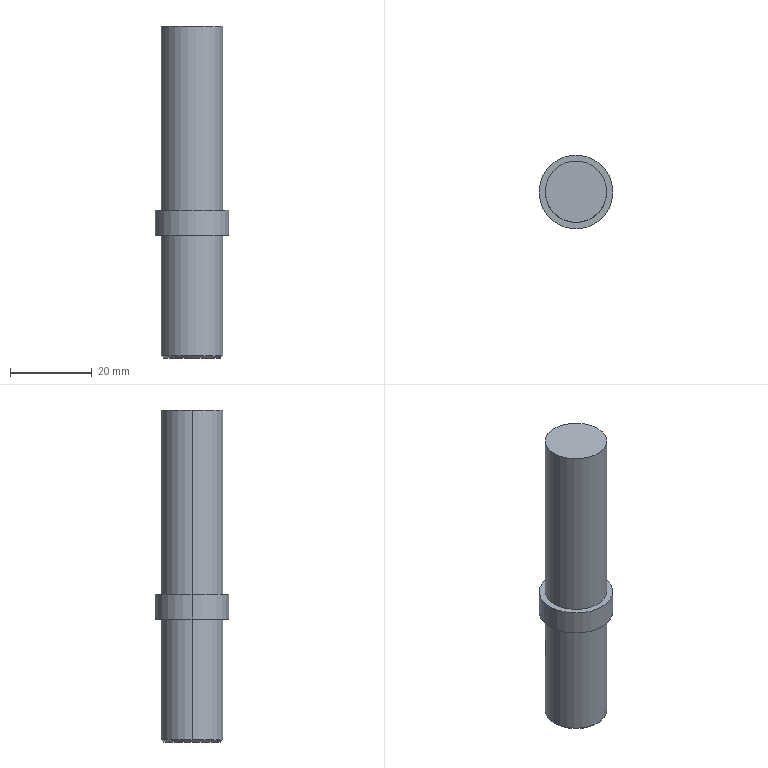Part | STEP file | 001-010-Waste driven wheel mounting shaft | 1 solid | 12 faces | box 18 x 18 x 81 mm | volume 14775 mm3 | cylinder 6 | plane 4 | cone 2 | commonest cylinder face diameters 15 x4 18 x2
STEP:
#1=CARTESIAN_POINT('',(0.,0.,0.));
#2=DIRECTION('',(0.,0.,1.));
#3=DIRECTION('',(1.,0.,0.));
#4=AXIS2_PLACEMENT_3D('',#1,#2,#3);
#5=CARTESIAN_POINT('',(-7.,0.,0.));
#6=VERTEX_POINT('',#5);
#7=CARTESIAN_POINT('',(7.,0.,0.));
#8=VERTEX_POINT('',#7);
#9=CARTESIAN_POINT('',(0.,0.,0.));
#10=DIRECTION('',(0.,0.,-1.));
#11=DIRECTION('',(1.,0.,0.));
#12=AXIS2_PLACEMENT_3D('',#9,#10,#11);
#13=CIRCLE('',#12,7.);
#14=CARTESIAN_POINT('',(0.,0.,0.5));
#15=DIRECTION('',(0.,0.,1.));
#16=DIRECTION('',(1.,0.,0.));
#17=AXIS2_PLACEMENT_3D('',#14,#15,#16);
#18=CONICAL_SURFACE('',#17,7.5,0.7854);
#19=CARTESIAN_POINT('',(6.283,-0.5));
#20=DIRECTION('',(-1.,0.));
#21=VECTOR('',#20,1.);
#22=LINE('',#19,#21);
#23=(GEOMETRIC_REPRESENTATION_CONTEXT(2)PARAMETRIC_REPRESENTATION_CONTEXT()REPRESENTATION_CONTEXT('',''));
#24=DEFINITIONAL_REPRESENTATION('',(#22),#23);
#25=PCURVE('',#18,#24);
#26=CARTESIAN_POINT('',(0.,0.,0.));
#27=DIRECTION('',(0.,0.,1.));
#28=DIRECTION('',(1.,0.,0.));
#29=AXIS2_PLACEMENT_3D('',#26,#27,#28);
#30=PLANE('',#29);
#31=CARTESIAN_POINT('',(7.,0.));
#32=CARTESIAN_POINT('',(7.,-12.124));
#33=CARTESIAN_POINT('',(-3.5,-6.062));
#34=CARTESIAN_POINT('',(-14.,0.));
#35=CARTESIAN_POINT('',(-3.5,6.062));
#36=CARTESIAN_POINT('',(7.,12.124));
#37=CARTESIAN_POINT('',(7.,0.));
#38=(BOUNDED_CURVE()B_SPLINE_CURVE(2,(#31,#32,#33,#34,#35,#36,#37),.UNSPECIFIED.,.T.,.F.)B_SPLINE_CURVE_WITH_KNOTS((1,2,2,2,2,1),(-2.094,0.,2.094,4.189,6.283,8.378),.UNSPECIFIED.)CURVE()GEOMETRIC_REPRESENTATION_ITEM()RATIONAL_B_SPLINE_CURVE((1.,0.5,1.,0.5,1.,0.5,1.))REPRESENTATION_ITEM(''));
#39=(GEOMETRIC_REPRESENTATION_CONTEXT(2)PARAMETRIC_REPRESENTATION_CONTEXT()REPRESENTATION_CONTEXT('',''));
#40=DEFINITIONAL_REPRESENTATION('',(#38),#39);
#41=PCURVE('',#30,#40);
#42=SURFACE_CURVE('',#13,(#25,#41),.PCURVE_S1.);
#43=EDGE_CURVE('',#6,#8,#42,.T.);
#44=ORIENTED_EDGE('',*,*,#43,.F.);
#45=CARTESIAN_POINT('',(-7.5,0.,0.5));
#46=VERTEX_POINT('',#45);
#47=CARTESIAN_POINT('',(-7.5,0.,0.5));
#48=DIRECTION('',(-0.7071,0.,0.7071));
#49=VECTOR('',#48,1.);
#50=LINE('',#47,#49);
#51=CARTESIAN_POINT('',(3.142,0.));
#52=DIRECTION('',(0.,1.));
#53=VECTOR('',#52,1.);
#54=LINE('',#51,#53);
#55=(GEOMETRIC_REPRESENTATION_CONTEXT(2)PARAMETRIC_REPRESENTATION_CONTEXT()REPRESENTATION_CONTEXT('',''));
#56=DEFINITIONAL_REPRESENTATION('',(#54),#55);
#57=PCURVE('',#18,#56);
#58=CARTESIAN_POINT('',(0.,0.,0.5));
#59=DIRECTION('',(0.,0.,1.));
#60=DIRECTION('',(1.,0.,0.));
#61=AXIS2_PLACEMENT_3D('',#58,#59,#60);
#62=CONICAL_SURFACE('',#61,7.5,0.7854);
#63=CARTESIAN_POINT('',(3.142,0.));
#64=DIRECTION('',(0.,1.));
#65=VECTOR('',#64,1.);
#66=LINE('',#63,#65);
#67=(GEOMETRIC_REPRESENTATION_CONTEXT(2)PARAMETRIC_REPRESENTATION_CONTEXT()REPRESENTATION_CONTEXT('',''));
#68=DEFINITIONAL_REPRESENTATION('',(#66),#67);
#69=PCURVE('',#62,#68);
#70=SURFACE_CURVE('',#50,(#57,#69),.PCURVE_S1.);
#71=EDGE_CURVE('',#6,#46,#70,.T.);
#72=ORIENTED_EDGE('',*,*,#71,.T.);
#73=CARTESIAN_POINT('',(7.5,0.,0.5));
#74=VERTEX_POINT('',#73);
#75=CARTESIAN_POINT('',(0.,0.,0.5));
#76=DIRECTION('',(0.,0.,1.));
#77=DIRECTION('',(1.,0.,0.));
#78=AXIS2_PLACEMENT_3D('',#75,#76,#77);
#79=CIRCLE('',#78,7.5);
#80=CARTESIAN_POINT('',(0.,0.));
#81=DIRECTION('',(1.,0.));
#82=VECTOR('',#81,1.);
#83=LINE('',#80,#82);
#84=(GEOMETRIC_REPRESENTATION_CONTEXT(2)PARAMETRIC_REPRESENTATION_CONTEXT()REPRESENTATION_CONTEXT('',''));
#85=DEFINITIONAL_REPRESENTATION('',(#83),#84);
#86=PCURVE('',#18,#85);
#87=CARTESIAN_POINT('',(0.,0.,30.));
#88=DIRECTION('',(0.,0.,-1.));
#89=DIRECTION('',(-1.,0.,0.));
#90=AXIS2_PLACEMENT_3D('',#87,#88,#89);
#91=CYLINDRICAL_SURFACE('',#90,7.5);
#92=CARTESIAN_POINT('',(3.142,29.5));
#93=DIRECTION('',(-1.,0.));
#94=VECTOR('',#93,1.);
#95=LINE('',#92,#94);
#96=(GEOMETRIC_REPRESENTATION_CONTEXT(2)PARAMETRIC_REPRESENTATION_CONTEXT()REPRESENTATION_CONTEXT('',''));
#97=DEFINITIONAL_REPRESENTATION('',(#95),#96);
#98=PCURVE('',#91,#97);
#99=SURFACE_CURVE('',#79,(#86,#98),.PCURVE_S1.);
#100=EDGE_CURVE('',#74,#46,#99,.T.);
#101=ORIENTED_EDGE('',*,*,#100,.F.);
#102=CARTESIAN_POINT('',(7.5,0.,0.5));
#103=DIRECTION('',(0.7071,0.,0.7071));
#104=VECTOR('',#103,1.);
#105=LINE('',#102,#104);
#106=CARTESIAN_POINT('',(0.,0.));
#107=DIRECTION('',(0.,1.));
#108=VECTOR('',#107,1.);
#109=LINE('',#106,#108);
#110=(GEOMETRIC_REPRESENTATION_CONTEXT(2)PARAMETRIC_REPRESENTATION_CONTEXT()REPRESENTATION_CONTEXT('',''));
#111=DEFINITIONAL_REPRESENTATION('',(#109),#110);
#112=PCURVE('',#18,#111);
#113=CARTESIAN_POINT('',(6.283,0.));
#114=DIRECTION('',(0.,1.));
#115=VECTOR('',#114,1.);
#116=LINE('',#113,#115);
#117=(GEOMETRIC_REPRESENTATION_CONTEXT(2)PARAMETRIC_REPRESENTATION_CONTEXT()REPRESENTATION_CONTEXT('',''));
#118=DEFINITIONAL_REPRESENTATION('',(#116),#117);
#119=PCURVE('',#62,#118);
#120=SURFACE_CURVE('',#105,(#112,#119),.PCURVE_S1.);
#121=EDGE_CURVE('',#8,#74,#120,.T.);
#122=ORIENTED_EDGE('',*,*,#121,.F.);
#123=EDGE_LOOP('',(#44,#72,#101,#122));
#124=FACE_BOUND('',#123,.T.);
#125=ADVANCED_FACE('',(#124),#18,.T.);
#126=CARTESIAN_POINT('',(7.5,0.,81.));
#127=VERTEX_POINT('',#126);
#128=CARTESIAN_POINT('',(-7.5,0.,81.));
#129=VERTEX_POINT('',#128);
#130=CARTESIAN_POINT('',(0.,0.,81.));
#131=DIRECTION('',(0.,0.,1.));
#132=DIRECTION('',(1.,0.,0.));
#133=AXIS2_PLACEMENT_3D('',#130,#131,#132);
#134=CIRCLE('',#133,7.5);
#135=CARTESIAN_POINT('',(0.,0.,81.));
#136=DIRECTION('',(0.,0.,-1.));
#137=DIRECTION('',(-1.,0.,0.));
#138=AXIS2_PLACEMENT_3D('',#135,#136,#137);
#139=CYLINDRICAL_SURFACE('',#138,7.5);
#140=CARTESIAN_POINT('',(3.142,0.));
#141=DIRECTION('',(-1.,0.));
#142=VECTOR('',#141,1.);
#143=LINE('',#140,#142);
#144=(GEOMETRIC_REPRESENTATION_CONTEXT(2)PARAMETRIC_REPRESENTATION_CONTEXT()REPRESENTATION_CONTEXT('',''));
#145=DEFINITIONAL_REPRESENTATION('',(#143),#144);
#146=PCURVE('',#139,#145);
#147=CARTESIAN_POINT('',(0.,0.,81.));
#148=DIRECTION('',(0.,0.,1.));
#149=DIRECTION('',(1.,0.,0.));
#150=AXIS2_PLACEMENT_3D('',#147,#148,#149);
#151=PLANE('',#150);
#152=CARTESIAN_POINT('',(0.,0.));
#153=DIRECTION('',(1.,0.));
#154=AXIS2_PLACEMENT_2D('',#152,#153);
#155=CIRCLE('',#154,7.5);
#156=(GEOMETRIC_REPRESENTATION_CONTEXT(2)PARAMETRIC_REPRESENTATION_CONTEXT()REPRESENTATION_CONTEXT('',''));
#157=DEFINITIONAL_REPRESENTATION('',(#155),#156);
#158=PCURVE('',#151,#157);
#159=SURFACE_CURVE('',#134,(#146,#158),.PCURVE_S1.);
#160=EDGE_CURVE('',#127,#129,#159,.T.);
#161=ORIENTED_EDGE('',*,*,#160,.F.);
#162=CARTESIAN_POINT('',(7.5,0.,36.));
#163=VERTEX_POINT('',#162);
#164=CARTESIAN_POINT('',(7.5,0.,81.));
#165=DIRECTION('',(0.,0.,-1.));
#166=VECTOR('',#165,1.);
#167=LINE('',#164,#166);
#168=CARTESIAN_POINT('',(3.142,0.));
#169=DIRECTION('',(0.,1.));
#170=VECTOR('',#169,1.);
#171=LINE('',#168,#170);
#172=(GEOMETRIC_REPRESENTATION_CONTEXT(2)PARAMETRIC_REPRESENTATION_CONTEXT()REPRESENTATION_CONTEXT('',''));
#173=DEFINITIONAL_REPRESENTATION('',(#171),#172);
#174=PCURVE('',#139,#173);
#175=CARTESIAN_POINT('',(0.,0.,81.));
#176=DIRECTION('',(0.,0.,-1.));
#177=DIRECTION('',(-1.,0.,0.));
#178=AXIS2_PLACEMENT_3D('',#175,#176,#177);
#179=CYLINDRICAL_SURFACE('',#178,7.5);
#180=CARTESIAN_POINT('',(3.142,0.));
#181=DIRECTION('',(0.,1.));
#182=VECTOR('',#181,1.);
#183=LINE('',#180,#182);
#184=(GEOMETRIC_REPRESENTATION_CONTEXT(2)PARAMETRIC_REPRESENTATION_CONTEXT()REPRESENTATION_CONTEXT('',''));
#185=DEFINITIONAL_REPRESENTATION('',(#183),#184);
#186=PCURVE('',#179,#185);
#187=SURFACE_CURVE('',#167,(#174,#186),.PCURVE_S1.);
#188=EDGE_CURVE('',#127,#163,#187,.T.);
#189=ORIENTED_EDGE('',*,*,#188,.T.);
#190=CARTESIAN_POINT('',(-7.5,0.,36.));
#191=VERTEX_POINT('',#190);
#192=CARTESIAN_POINT('',(0.,0.,36.));
#193=DIRECTION('',(0.,0.,1.));
#194=DIRECTION('',(1.,0.,0.));
#195=AXIS2_PLACEMENT_3D('',#192,#193,#194);
#196=CIRCLE('',#195,7.5);
#197=CARTESIAN_POINT('',(3.142,45.));
#198=DIRECTION('',(-1.,0.));
#199=VECTOR('',#198,1.);
#200=LINE('',#197,#199);
#201=(GEOMETRIC_REPRESENTATION_CONTEXT(2)PARAMETRIC_REPRESENTATION_CONTEXT()REPRESENTATION_CONTEXT('',''));
#202=DEFINITIONAL_REPRESENTATION('',(#200),#201);
#203=PCURVE('',#139,#202);
#204=CARTESIAN_POINT('',(0.,0.,36.));
#205=DIRECTION('',(0.,0.,1.));
#206=DIRECTION('',(1.,0.,0.));
#207=AXIS2_PLACEMENT_3D('',#204,#205,#206);
#208=PLANE('',#207);
#209=CARTESIAN_POINT('',(0.,0.));
#210=DIRECTION('',(1.,0.));
#211=AXIS2_PLACEMENT_2D('',#209,#210);
#212=CIRCLE('',#211,7.5);
#213=(GEOMETRIC_REPRESENTATION_CONTEXT(2)PARAMETRIC_REPRESENTATION_CONTEXT()REPRESENTATION_CONTEXT('',''));
#214=DEFINITIONAL_REPRESENTATION('',(#212),#213);
#215=PCURVE('',#208,#214);
#216=SURFACE_CURVE('',#196,(#203,#215),.PCURVE_S1.);
#217=EDGE_CURVE('',#163,#191,#216,.T.);
#218=ORIENTED_EDGE('',*,*,#217,.T.);
#219=CARTESIAN_POINT('',(-7.5,0.,81.));
#220=DIRECTION('',(0.,0.,-1.));
#221=VECTOR('',#220,1.);
#222=LINE('',#219,#221);
#223=CARTESIAN_POINT('',(0.,0.));
#224=DIRECTION('',(0.,1.));
#225=VECTOR('',#224,1.);
#226=LINE('',#223,#225);
#227=(GEOMETRIC_REPRESENTATION_CONTEXT(2)PARAMETRIC_REPRESENTATION_CONTEXT()REPRESENTATION_CONTEXT('',''));
#228=DEFINITIONAL_REPRESENTATION('',(#226),#227);
#229=PCURVE('',#139,#228);
#230=CARTESIAN_POINT('',(6.283,0.));
#231=DIRECTION('',(0.,1.));
#232=VECTOR('',#231,1.);
#233=LINE('',#230,#232);
#234=(GEOMETRIC_REPRESENTATION_CONTEXT(2)PARAMETRIC_REPRESENTATION_CONTEXT()REPRESENTATION_CONTEXT('',''));
#235=DEFINITIONAL_REPRESENTATION('',(#233),#234);
#236=PCURVE('',#179,#235);
#237=SURFACE_CURVE('',#222,(#229,#236),.PCURVE_S1.);
#238=EDGE_CURVE('',#129,#191,#237,.T.);
#239=ORIENTED_EDGE('',*,*,#238,.F.);
#240=EDGE_LOOP('',(#161,#189,#218,#239));
#241=FACE_BOUND('',#240,.T.);
#242=ADVANCED_FACE('',(#241),#139,.T.);
#243=CARTESIAN_POINT('',(9.,0.,36.));
#244=VERTEX_POINT('',#243);
#245=CARTESIAN_POINT('',(-9.,0.,36.));
#246=VERTEX_POINT('',#245);
#247=CARTESIAN_POINT('',(0.,0.,36.));
#248=DIRECTION('',(0.,0.,1.));
#249=DIRECTION('',(1.,0.,0.));
#250=AXIS2_PLACEMENT_3D('',#247,#248,#249);
#251=CIRCLE('',#250,9.);
#252=CARTESIAN_POINT('',(0.,0.,36.));
#253=DIRECTION('',(0.,0.,-1.));
#254=DIRECTION('',(-1.,0.,0.));
#255=AXIS2_PLACEMENT_3D('',#252,#253,#254);
#256=CYLINDRICAL_SURFACE('',#255,9.);
#257=CARTESIAN_POINT('',(3.142,0.));
#258=DIRECTION('',(-1.,0.));
#259=VECTOR('',#258,1.);
#260=LINE('',#257,#259);
#261=(GEOMETRIC_REPRESENTATION_CONTEXT(2)PARAMETRIC_REPRESENTATION_CONTEXT()REPRESENTATION_CONTEXT('',''));
#262=DEFINITIONAL_REPRESENTATION('',(#260),#261);
#263=PCURVE('',#256,#262);
#264=CARTESIAN_POINT('',(0.,0.));
#265=DIRECTION('',(1.,0.));
#266=AXIS2_PLACEMENT_2D('',#264,#265);
#267=CIRCLE('',#266,9.);
#268=(GEOMETRIC_REPRESENTATION_CONTEXT(2)PARAMETRIC_REPRESENTATION_CONTEXT()REPRESENTATION_CONTEXT('',''));
#269=DEFINITIONAL_REPRESENTATION('',(#267),#268);
#270=PCURVE('',#208,#269);
#271=SURFACE_CURVE('',#251,(#263,#270),.PCURVE_S1.);
#272=EDGE_CURVE('',#244,#246,#271,.T.);
#273=ORIENTED_EDGE('',*,*,#272,.F.);
#274=CARTESIAN_POINT('',(9.,0.,30.));
#275=VERTEX_POINT('',#274);
#276=CARTESIAN_POINT('',(9.,0.,36.));
#277=DIRECTION('',(0.,0.,-1.));
#278=VECTOR('',#277,1.);
#279=LINE('',#276,#278);
#280=CARTESIAN_POINT('',(3.142,0.));
#281=DIRECTION('',(0.,1.));
#282=VECTOR('',#281,1.);
#283=LINE('',#280,#282);
#284=(GEOMETRIC_REPRESENTATION_CONTEXT(2)PARAMETRIC_REPRESENTATION_CONTEXT()REPRESENTATION_CONTEXT('',''));
#285=DEFINITIONAL_REPRESENTATION('',(#283),#284);
#286=PCURVE('',#256,#285);
#287=CARTESIAN_POINT('',(0.,0.,36.));
#288=DIRECTION('',(0.,0.,-1.));
#289=DIRECTION('',(-1.,0.,0.));
#290=AXIS2_PLACEMENT_3D('',#287,#288,#289);
#291=CYLINDRICAL_SURFACE('',#290,9.);
#292=CARTESIAN_POINT('',(3.142,0.));
#293=DIRECTION('',(0.,1.));
#294=VECTOR('',#293,1.);
#295=LINE('',#292,#294);
#296=(GEOMETRIC_REPRESENTATION_CONTEXT(2)PARAMETRIC_REPRESENTATION_CONTEXT()REPRESENTATION_CONTEXT('',''));
#297=DEFINITIONAL_REPRESENTATION('',(#295),#296);
#298=PCURVE('',#291,#297);
#299=SURFACE_CURVE('',#279,(#286,#298),.PCURVE_S1.);
#300=EDGE_CURVE('',#244,#275,#299,.T.);
#301=ORIENTED_EDGE('',*,*,#300,.T.);
#302=CARTESIAN_POINT('',(-9.,0.,30.));
#303=VERTEX_POINT('',#302);
#304=CARTESIAN_POINT('',(0.,0.,30.));
#305=DIRECTION('',(0.,0.,1.));
#306=DIRECTION('',(1.,0.,0.));
#307=AXIS2_PLACEMENT_3D('',#304,#305,#306);
#308=CIRCLE('',#307,9.);
#309=CARTESIAN_POINT('',(3.142,6.));
#310=DIRECTION('',(-1.,0.));
#311=VECTOR('',#310,1.);
#312=LINE('',#309,#311);
#313=(GEOMETRIC_REPRESENTATION_CONTEXT(2)PARAMETRIC_REPRESENTATION_CONTEXT()REPRESENTATION_CONTEXT('',''));
#314=DEFINITIONAL_REPRESENTATION('',(#312),#313);
#315=PCURVE('',#256,#314);
#316=CARTESIAN_POINT('',(0.,0.,30.));
#317=DIRECTION('',(0.,0.,1.));
#318=DIRECTION('',(1.,0.,0.));
#319=AXIS2_PLACEMENT_3D('',#316,#317,#318);
#320=PLANE('',#319);
#321=CARTESIAN_POINT('',(0.,0.));
#322=DIRECTION('',(1.,0.));
#323=AXIS2_PLACEMENT_2D('',#321,#322);
#324=CIRCLE('',#323,9.);
#325=(GEOMETRIC_REPRESENTATION_CONTEXT(2)PARAMETRIC_REPRESENTATION_CONTEXT()REPRESENTATION_CONTEXT('',''));
#326=DEFINITIONAL_REPRESENTATION('',(#324),#325);
#327=PCURVE('',#320,#326);
#328=SURFACE_CURVE('',#308,(#315,#327),.PCURVE_S1.);
#329=EDGE_CURVE('',#275,#303,#328,.T.);
#330=ORIENTED_EDGE('',*,*,#329,.T.);
#331=CARTESIAN_POINT('',(-9.,0.,36.));
#332=DIRECTION('',(0.,0.,-1.));
#333=VECTOR('',#332,1.);
#334=LINE('',#331,#333);
#335=CARTESIAN_POINT('',(0.,0.));
#336=DIRECTION('',(0.,1.));
#337=VECTOR('',#336,1.);
#338=LINE('',#335,#337);
#339=(GEOMETRIC_REPRESENTATION_CONTEXT(2)PARAMETRIC_REPRESENTATION_CONTEXT()REPRESENTATION_CONTEXT('',''));
#340=DEFINITIONAL_REPRESENTATION('',(#338),#339);
#341=PCURVE('',#256,#340);
#342=CARTESIAN_POINT('',(6.283,0.));
#343=DIRECTION('',(0.,1.));
#344=VECTOR('',#343,1.);
#345=LINE('',#342,#344);
#346=(GEOMETRIC_REPRESENTATION_CONTEXT(2)PARAMETRIC_REPRESENTATION_CONTEXT()REPRESENTATION_CONTEXT('',''));
#347=DEFINITIONAL_REPRESENTATION('',(#345),#346);
#348=PCURVE('',#291,#347);
#349=SURFACE_CURVE('',#334,(#341,#348),.PCURVE_S1.);
#350=EDGE_CURVE('',#246,#303,#349,.T.);
#351=ORIENTED_EDGE('',*,*,#350,.F.);
#352=EDGE_LOOP('',(#273,#301,#330,#351));
#353=FACE_BOUND('',#352,.T.);
#354=ADVANCED_FACE('',(#353),#256,.T.);
#355=CARTESIAN_POINT('',(7.5,0.,30.));
#356=VERTEX_POINT('',#355);
#357=CARTESIAN_POINT('',(-7.5,0.,30.));
#358=VERTEX_POINT('',#357);
#359=CARTESIAN_POINT('',(0.,0.,30.));
#360=DIRECTION('',(0.,0.,1.));
#361=DIRECTION('',(1.,0.,0.));
#362=AXIS2_PLACEMENT_3D('',#359,#360,#361);
#363=CIRCLE('',#362,7.5);
#364=CARTESIAN_POINT('',(3.142,0.));
#365=DIRECTION('',(-1.,0.));
#366=VECTOR('',#365,1.);
#367=LINE('',#364,#366);
#368=(GEOMETRIC_REPRESENTATION_CONTEXT(2)PARAMETRIC_REPRESENTATION_CONTEXT()REPRESENTATION_CONTEXT('',''));
#369=DEFINITIONAL_REPRESENTATION('',(#367),#368);
#370=PCURVE('',#91,#369);
#371=CARTESIAN_POINT('',(0.,0.));
#372=DIRECTION('',(1.,0.));
#373=AXIS2_PLACEMENT_2D('',#371,#372);
#374=CIRCLE('',#373,7.5);
#375=(GEOMETRIC_REPRESENTATION_CONTEXT(2)PARAMETRIC_REPRESENTATION_CONTEXT()REPRESENTATION_CONTEXT('',''));
#376=DEFINITIONAL_REPRESENTATION('',(#374),#375);
#377=PCURVE('',#320,#376);
#378=SURFACE_CURVE('',#363,(#370,#377),.PCURVE_S1.);
#379=EDGE_CURVE('',#356,#358,#378,.T.);
#380=ORIENTED_EDGE('',*,*,#379,.F.);
#381=CARTESIAN_POINT('',(7.5,0.,30.));
#382=DIRECTION('',(0.,0.,-1.));
#383=VECTOR('',#382,1.);
#384=LINE('',#381,#383);
#385=CARTESIAN_POINT('',(3.142,0.));
#386=DIRECTION('',(0.,1.));
#387=VECTOR('',#386,1.);
#388=LINE('',#385,#387);
#389=(GEOMETRIC_REPRESENTATION_CONTEXT(2)PARAMETRIC_REPRESENTATION_CONTEXT()REPRESENTATION_CONTEXT('',''));
#390=DEFINITIONAL_REPRESENTATION('',(#388),#389);
#391=PCURVE('',#91,#390);
#392=CARTESIAN_POINT('',(0.,0.,30.));
#393=DIRECTION('',(0.,0.,-1.));
#394=DIRECTION('',(-1.,0.,0.));
#395=AXIS2_PLACEMENT_3D('',#392,#393,#394);
#396=CYLINDRICAL_SURFACE('',#395,7.5);
#397=CARTESIAN_POINT('',(3.142,0.));
#398=DIRECTION('',(0.,1.));
#399=VECTOR('',#398,1.);
#400=LINE('',#397,#399);
#401=(GEOMETRIC_REPRESENTATION_CONTEXT(2)PARAMETRIC_REPRESENTATION_CONTEXT()REPRESENTATION_CONTEXT('',''));
#402=DEFINITIONAL_REPRESENTATION('',(#400),#401);
#403=PCURVE('',#396,#402);
#404=SURFACE_CURVE('',#384,(#391,#403),.PCURVE_S1.);
#405=EDGE_CURVE('',#356,#74,#404,.T.);
#406=ORIENTED_EDGE('',*,*,#405,.T.);
#407=ORIENTED_EDGE('',*,*,#100,.T.);
#408=CARTESIAN_POINT('',(-7.5,0.,30.));
#409=DIRECTION('',(0.,0.,-1.));
#410=VECTOR('',#409,1.);
#411=LINE('',#408,#410);
#412=CARTESIAN_POINT('',(0.,0.));
#413=DIRECTION('',(0.,1.));
#414=VECTOR('',#413,1.);
#415=LINE('',#412,#414);
#416=(GEOMETRIC_REPRESENTATION_CONTEXT(2)PARAMETRIC_REPRESENTATION_CONTEXT()REPRESENTATION_CONTEXT('',''));
#417=DEFINITIONAL_REPRESENTATION('',(#415),#416);
#418=PCURVE('',#91,#417);
#419=CARTESIAN_POINT('',(6.283,0.));
#420=DIRECTION('',(0.,1.));
#421=VECTOR('',#420,1.);
#422=LINE('',#419,#421);
#423=(GEOMETRIC_REPRESENTATION_CONTEXT(2)PARAMETRIC_REPRESENTATION_CONTEXT()REPRESENTATION_CONTEXT('',''));
#424=DEFINITIONAL_REPRESENTATION('',(#422),#423);
#425=PCURVE('',#396,#424);
#426=SURFACE_CURVE('',#411,(#418,#425),.PCURVE_S1.);
#427=EDGE_CURVE('',#358,#46,#426,.T.);
#428=ORIENTED_EDGE('',*,*,#427,.F.);
#429=EDGE_LOOP('',(#380,#406,#407,#428));
#430=FACE_BOUND('',#429,.T.);
#431=ADVANCED_FACE('',(#430),#91,.T.);
#432=ORIENTED_EDGE('',*,*,#405,.F.);
#433=CARTESIAN_POINT('',(0.,0.,30.));
#434=DIRECTION('',(0.,0.,1.));
#435=DIRECTION('',(1.,0.,0.));
#436=AXIS2_PLACEMENT_3D('',#433,#434,#435);
#437=CIRCLE('',#436,7.5);
#438=CARTESIAN_POINT('',(9.425,0.));
#439=DIRECTION('',(-1.,0.));
#440=VECTOR('',#439,1.);
#441=LINE('',#438,#440);
#442=(GEOMETRIC_REPRESENTATION_CONTEXT(2)PARAMETRIC_REPRESENTATION_CONTEXT()REPRESENTATION_CONTEXT('',''));
#443=DEFINITIONAL_REPRESENTATION('',(#441),#442);
#444=PCURVE('',#396,#443);
#445=CARTESIAN_POINT('',(0.,0.));
#446=DIRECTION('',(1.,0.));
#447=AXIS2_PLACEMENT_2D('',#445,#446);
#448=CIRCLE('',#447,7.5);
#449=(GEOMETRIC_REPRESENTATION_CONTEXT(2)PARAMETRIC_REPRESENTATION_CONTEXT()REPRESENTATION_CONTEXT('',''));
#450=DEFINITIONAL_REPRESENTATION('',(#448),#449);
#451=PCURVE('',#320,#450);
#452=SURFACE_CURVE('',#437,(#444,#451),.PCURVE_S1.);
#453=EDGE_CURVE('',#358,#356,#452,.T.);
#454=ORIENTED_EDGE('',*,*,#453,.F.);
#455=ORIENTED_EDGE('',*,*,#427,.T.);
#456=CARTESIAN_POINT('',(0.,0.,0.5));
#457=DIRECTION('',(0.,0.,1.));
#458=DIRECTION('',(1.,0.,0.));
#459=AXIS2_PLACEMENT_3D('',#456,#457,#458);
#460=CIRCLE('',#459,7.5);
#461=CARTESIAN_POINT('',(9.425,29.5));
#462=DIRECTION('',(-1.,0.));
#463=VECTOR('',#462,1.);
#464=LINE('',#461,#463);
#465=(GEOMETRIC_REPRESENTATION_CONTEXT(2)PARAMETRIC_REPRESENTATION_CONTEXT()REPRESENTATION_CONTEXT('',''));
#466=DEFINITIONAL_REPRESENTATION('',(#464),#465);
#467=PCURVE('',#396,#466);
#468=CARTESIAN_POINT('',(0.,0.));
#469=DIRECTION('',(1.,0.));
#470=VECTOR('',#469,1.);
#471=LINE('',#468,#470);
#472=(GEOMETRIC_REPRESENTATION_CONTEXT(2)PARAMETRIC_REPRESENTATION_CONTEXT()REPRESENTATION_CONTEXT('',''));
#473=DEFINITIONAL_REPRESENTATION('',(#471),#472);
#474=PCURVE('',#62,#473);
#475=SURFACE_CURVE('',#460,(#467,#474),.PCURVE_S1.);
#476=EDGE_CURVE('',#46,#74,#475,.T.);
#477=ORIENTED_EDGE('',*,*,#476,.T.);
#478=EDGE_LOOP('',(#432,#454,#455,#477));
#479=FACE_BOUND('',#478,.T.);
#480=ADVANCED_FACE('',(#479),#396,.T.);
#481=CARTESIAN_POINT('',(0.,0.,0.));
#482=DIRECTION('',(0.,0.,-1.));
#483=DIRECTION('',(1.,0.,0.));
#484=AXIS2_PLACEMENT_3D('',#481,#482,#483);
#485=CIRCLE('',#484,7.);
#486=CARTESIAN_POINT('',(7.,0.));
#487=CARTESIAN_POINT('',(7.,-12.124));
#488=CARTESIAN_POINT('',(-3.5,-6.062));
#489=CARTESIAN_POINT('',(-14.,0.));
#490=CARTESIAN_POINT('',(-3.5,6.062));
#491=CARTESIAN_POINT('',(7.,12.124));
#492=CARTESIAN_POINT('',(7.,0.));
#493=(BOUNDED_CURVE()B_SPLINE_CURVE(2,(#486,#487,#488,#489,#490,#491,#492),.UNSPECIFIED.,.T.,.F.)B_SPLINE_CURVE_WITH_KNOTS((1,2,2,2,2,1),(-2.094,0.,2.094,4.189,6.283,8.378),.UNSPECIFIED.)CURVE()GEOMETRIC_REPRESENTATION_ITEM()RATIONAL_B_SPLINE_CURVE((1.,0.5,1.,0.5,1.,0.5,1.))REPRESENTATION_ITEM(''));
#494=(GEOMETRIC_REPRESENTATION_CONTEXT(2)PARAMETRIC_REPRESENTATION_CONTEXT()REPRESENTATION_CONTEXT('',''));
#495=DEFINITIONAL_REPRESENTATION('',(#493),#494);
#496=PCURVE('',#30,#495);
#497=CARTESIAN_POINT('',(6.283,-0.5));
#498=DIRECTION('',(-1.,0.));
#499=VECTOR('',#498,1.);
#500=LINE('',#497,#499);
#501=(GEOMETRIC_REPRESENTATION_CONTEXT(2)PARAMETRIC_REPRESENTATION_CONTEXT()REPRESENTATION_CONTEXT('',''));
#502=DEFINITIONAL_REPRESENTATION('',(#500),#501);
#503=PCURVE('',#62,#502);
#504=SURFACE_CURVE('',#485,(#496,#503),.PCURVE_S1.);
#505=EDGE_CURVE('',#8,#6,#504,.T.);
#506=ORIENTED_EDGE('',*,*,#505,.T.);
#507=ORIENTED_EDGE('',*,*,#43,.T.);
#508=EDGE_LOOP('',(#506,#507));
#509=FACE_BOUND('',#508,.T.);
#510=ADVANCED_FACE('',(#509),#30,.F.);
#511=ORIENTED_EDGE('',*,*,#300,.F.);
#512=CARTESIAN_POINT('',(0.,0.,36.));
#513=DIRECTION('',(0.,0.,1.));
#514=DIRECTION('',(1.,0.,0.));
#515=AXIS2_PLACEMENT_3D('',#512,#513,#514);
#516=CIRCLE('',#515,9.);
#517=CARTESIAN_POINT('',(9.425,0.));
#518=DIRECTION('',(-1.,0.));
#519=VECTOR('',#518,1.);
#520=LINE('',#517,#519);
#521=(GEOMETRIC_REPRESENTATION_CONTEXT(2)PARAMETRIC_REPRESENTATION_CONTEXT()REPRESENTATION_CONTEXT('',''));
#522=DEFINITIONAL_REPRESENTATION('',(#520),#521);
#523=PCURVE('',#291,#522);
#524=CARTESIAN_POINT('',(0.,0.));
#525=DIRECTION('',(1.,0.));
#526=AXIS2_PLACEMENT_2D('',#524,#525);
#527=CIRCLE('',#526,9.);
#528=(GEOMETRIC_REPRESENTATION_CONTEXT(2)PARAMETRIC_REPRESENTATION_CONTEXT()REPRESENTATION_CONTEXT('',''));
#529=DEFINITIONAL_REPRESENTATION('',(#527),#528);
#530=PCURVE('',#208,#529);
#531=SURFACE_CURVE('',#516,(#523,#530),.PCURVE_S1.);
#532=EDGE_CURVE('',#246,#244,#531,.T.);
#533=ORIENTED_EDGE('',*,*,#532,.F.);
#534=ORIENTED_EDGE('',*,*,#350,.T.);
#535=CARTESIAN_POINT('',(0.,0.,30.));
#536=DIRECTION('',(0.,0.,1.));
#537=DIRECTION('',(1.,0.,0.));
#538=AXIS2_PLACEMENT_3D('',#535,#536,#537);
#539=CIRCLE('',#538,9.);
#540=CARTESIAN_POINT('',(9.425,6.));
#541=DIRECTION('',(-1.,0.));
#542=VECTOR('',#541,1.);
#543=LINE('',#540,#542);
#544=(GEOMETRIC_REPRESENTATION_CONTEXT(2)PARAMETRIC_REPRESENTATION_CONTEXT()REPRESENTATION_CONTEXT('',''));
#545=DEFINITIONAL_REPRESENTATION('',(#543),#544);
#546=PCURVE('',#291,#545);
#547=CARTESIAN_POINT('',(0.,0.));
#548=DIRECTION('',(1.,0.));
#549=AXIS2_PLACEMENT_2D('',#547,#548);
#550=CIRCLE('',#549,9.);
#551=(GEOMETRIC_REPRESENTATION_CONTEXT(2)PARAMETRIC_REPRESENTATION_CONTEXT()REPRESENTATION_CONTEXT('',''));
#552=DEFINITIONAL_REPRESENTATION('',(#550),#551);
#553=PCURVE('',#320,#552);
#554=SURFACE_CURVE('',#539,(#546,#553),.PCURVE_S1.);
#555=EDGE_CURVE('',#303,#275,#554,.T.);
#556=ORIENTED_EDGE('',*,*,#555,.T.);
#557=EDGE_LOOP('',(#511,#533,#534,#556));
#558=FACE_BOUND('',#557,.T.);
#559=ADVANCED_FACE('',(#558),#291,.T.);
#560=CARTESIAN_POINT('',(0.,0.,36.));
#561=DIRECTION('',(0.,0.,1.));
#562=DIRECTION('',(1.,0.,0.));
#563=AXIS2_PLACEMENT_3D('',#560,#561,#562);
#564=CIRCLE('',#563,7.5);
#565=CARTESIAN_POINT('',(0.,0.));
#566=DIRECTION('',(1.,0.));
#567=AXIS2_PLACEMENT_2D('',#565,#566);
#568=CIRCLE('',#567,7.5);
#569=(GEOMETRIC_REPRESENTATION_CONTEXT(2)PARAMETRIC_REPRESENTATION_CONTEXT()REPRESENTATION_CONTEXT('',''));
#570=DEFINITIONAL_REPRESENTATION('',(#568),#569);
#571=PCURVE('',#208,#570);
#572=CARTESIAN_POINT('',(9.425,45.));
#573=DIRECTION('',(-1.,0.));
#574=VECTOR('',#573,1.);
#575=LINE('',#572,#574);
#576=(GEOMETRIC_REPRESENTATION_CONTEXT(2)PARAMETRIC_REPRESENTATION_CONTEXT()REPRESENTATION_CONTEXT('',''));
#577=DEFINITIONAL_REPRESENTATION('',(#575),#576);
#578=PCURVE('',#179,#577);
#579=SURFACE_CURVE('',#564,(#571,#578),.PCURVE_S1.);
#580=EDGE_CURVE('',#191,#163,#579,.T.);
#581=ORIENTED_EDGE('',*,*,#580,.F.);
#582=ORIENTED_EDGE('',*,*,#217,.F.);
#583=EDGE_LOOP('',(#581,#582));
#584=FACE_BOUND('',#583,.T.);
#585=ORIENTED_EDGE('',*,*,#532,.T.);
#586=ORIENTED_EDGE('',*,*,#272,.T.);
#587=EDGE_LOOP('',(#585,#586));
#588=FACE_BOUND('',#587,.T.);
#589=ADVANCED_FACE('',(#584,#588),#208,.T.);
#590=ORIENTED_EDGE('',*,*,#453,.T.);
#591=ORIENTED_EDGE('',*,*,#379,.T.);
#592=EDGE_LOOP('',(#590,#591));
#593=FACE_BOUND('',#592,.T.);
#594=ORIENTED_EDGE('',*,*,#555,.F.);
#595=ORIENTED_EDGE('',*,*,#329,.F.);
#596=EDGE_LOOP('',(#594,#595));
#597=FACE_BOUND('',#596,.T.);
#598=ADVANCED_FACE('',(#593,#597),#320,.F.);
#599=ORIENTED_EDGE('',*,*,#188,.F.);
#600=CARTESIAN_POINT('',(0.,0.,81.));
#601=DIRECTION('',(0.,0.,1.));
#602=DIRECTION('',(1.,0.,0.));
#603=AXIS2_PLACEMENT_3D('',#600,#601,#602);
#604=CIRCLE('',#603,7.5);
#605=CARTESIAN_POINT('',(9.425,0.));
#606=DIRECTION('',(-1.,0.));
#607=VECTOR('',#606,1.);
#608=LINE('',#605,#607);
#609=(GEOMETRIC_REPRESENTATION_CONTEXT(2)PARAMETRIC_REPRESENTATION_CONTEXT()REPRESENTATION_CONTEXT('',''));
#610=DEFINITIONAL_REPRESENTATION('',(#608),#609);
#611=PCURVE('',#179,#610);
#612=CARTESIAN_POINT('',(0.,0.));
#613=DIRECTION('',(1.,0.));
#614=AXIS2_PLACEMENT_2D('',#612,#613);
#615=CIRCLE('',#614,7.5);
#616=(GEOMETRIC_REPRESENTATION_CONTEXT(2)PARAMETRIC_REPRESENTATION_CONTEXT()REPRESENTATION_CONTEXT('',''));
#617=DEFINITIONAL_REPRESENTATION('',(#615),#616);
#618=PCURVE('',#151,#617);
#619=SURFACE_CURVE('',#604,(#611,#618),.PCURVE_S1.);
#620=EDGE_CURVE('',#129,#127,#619,.T.);
#621=ORIENTED_EDGE('',*,*,#620,.F.);
#622=ORIENTED_EDGE('',*,*,#238,.T.);
#623=ORIENTED_EDGE('',*,*,#580,.T.);
#624=EDGE_LOOP('',(#599,#621,#622,#623));
#625=FACE_BOUND('',#624,.T.);
#626=ADVANCED_FACE('',(#625),#179,.T.);
#627=ORIENTED_EDGE('',*,*,#620,.T.);
#628=ORIENTED_EDGE('',*,*,#160,.T.);
#629=EDGE_LOOP('',(#627,#628));
#630=FACE_BOUND('',#629,.T.);
#631=ADVANCED_FACE('',(#630),#151,.T.);
#632=ORIENTED_EDGE('',*,*,#71,.F.);
#633=ORIENTED_EDGE('',*,*,#505,.F.);
#634=ORIENTED_EDGE('',*,*,#121,.T.);
#635=ORIENTED_EDGE('',*,*,#476,.F.);
#636=EDGE_LOOP('',(#632,#633,#634,#635));
#637=FACE_BOUND('',#636,.T.);
#638=ADVANCED_FACE('',(#637),#62,.T.);
#639=CLOSED_SHELL('',(#125,#242,#354,#431,#480,#510,#559,#589,#598,#626,#631,#638));
#640=MANIFOLD_SOLID_BREP('',#639);
#641=(LENGTH_UNIT()NAMED_UNIT(*)SI_UNIT(.MILLI.,.METRE.));
#642=UNCERTAINTY_MEASURE_WITH_UNIT(LENGTH_MEASURE(0.0000001),#641,'','');
#643=(NAMED_UNIT(*)PLANE_ANGLE_UNIT()SI_UNIT($,.RADIAN.));
#644=(NAMED_UNIT(*)SI_UNIT($,.STERADIAN.)SOLID_ANGLE_UNIT());
#645=(GEOMETRIC_REPRESENTATION_CONTEXT(3)GLOBAL_UNCERTAINTY_ASSIGNED_CONTEXT((#642))GLOBAL_UNIT_ASSIGNED_CONTEXT((#641,#643,#644))REPRESENTATION_CONTEXT('',''));
#646=ADVANCED_BREP_SHAPE_REPRESENTATION('',(#4,#640),#645);